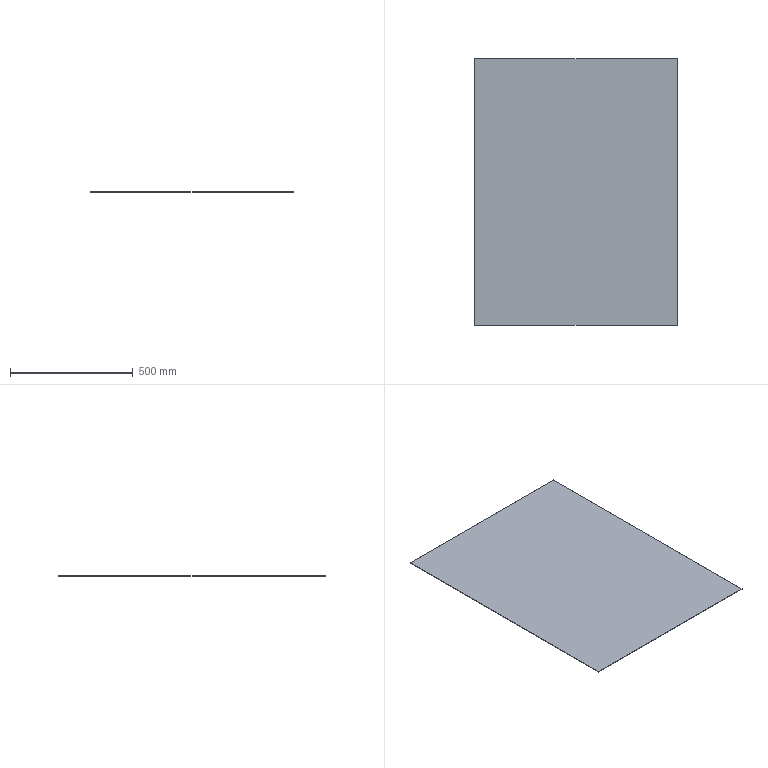Part | STEP file | Guide wheel mechanism revised.sldasm-Part-20 | 1 solid | 6 faces | box 825 x 1085 x 2 mm | volume 1790250 mm3 | plane 6
STEP:
#1=CARTESIAN_POINT('',(-412.5,812.5,-509.));
#2=VERTEX_POINT('',#1);
#3=CARTESIAN_POINT('',(-412.5,1897.5,-509.));
#4=VERTEX_POINT('',#3);
#5=CARTESIAN_POINT('',(-412.5,1897.5,-509.));
#6=DIRECTION('',(0.,1.,0.));
#7=VECTOR('',#6,1000.);
#8=LINE('',#5,#7);
#9=EDGE_CURVE('',#2,#4,#8,.T.);
#10=ORIENTED_EDGE('',*,*,#9,.T.);
#11=CARTESIAN_POINT('',(-412.5,1897.5,-511.));
#12=VERTEX_POINT('',#11);
#13=CARTESIAN_POINT('',(-412.5,1897.5,-511.));
#14=DIRECTION('',(0.,0.,1.));
#15=VECTOR('',#14,1000.);
#16=LINE('',#13,#15);
#17=EDGE_CURVE('',#12,#4,#16,.T.);
#18=ORIENTED_EDGE('',*,*,#17,.F.);
#19=CARTESIAN_POINT('',(-412.5,812.5,-511.));
#20=VERTEX_POINT('',#19);
#21=CARTESIAN_POINT('',(-412.5,1897.5,-511.));
#22=DIRECTION('',(0.,1.,0.));
#23=VECTOR('',#22,1000.);
#24=LINE('',#21,#23);
#25=EDGE_CURVE('',#20,#12,#24,.T.);
#26=ORIENTED_EDGE('',*,*,#25,.F.);
#27=CARTESIAN_POINT('',(-412.5,812.5,-511.));
#28=DIRECTION('',(0.,0.,1.));
#29=VECTOR('',#28,1000.);
#30=LINE('',#27,#29);
#31=EDGE_CURVE('',#20,#2,#30,.T.);
#32=ORIENTED_EDGE('',*,*,#31,.T.);
#33=EDGE_LOOP('',(#10,#18,#26,#32));
#34=FACE_OUTER_BOUND('',#33,.T.);
#35=CARTESIAN_POINT('',(-412.5,1897.5,-511.));
#36=DIRECTION('',(1.,0.,0.));
#37=DIRECTION('',(0.,1.,0.));
#38=AXIS2_PLACEMENT_3D('',#35,#36,#37);
#39=PLANE('',#38);
#40=ADVANCED_FACE('',(#34),#39,.F.);
#41=CARTESIAN_POINT('',(412.5,1897.5,-509.));
#42=VERTEX_POINT('',#41);
#43=CARTESIAN_POINT('',(-412.5,1897.5,-509.));
#44=DIRECTION('',(1.,0.,0.));
#45=VECTOR('',#44,1000.);
#46=LINE('',#43,#45);
#47=EDGE_CURVE('',#4,#42,#46,.T.);
#48=ORIENTED_EDGE('',*,*,#47,.T.);
#49=CARTESIAN_POINT('',(412.5,1897.5,-511.));
#50=VERTEX_POINT('',#49);
#51=CARTESIAN_POINT('',(412.5,1897.5,-511.));
#52=DIRECTION('',(0.,0.,1.));
#53=VECTOR('',#52,1000.);
#54=LINE('',#51,#53);
#55=EDGE_CURVE('',#50,#42,#54,.T.);
#56=ORIENTED_EDGE('',*,*,#55,.F.);
#57=CARTESIAN_POINT('',(-412.5,1897.5,-511.));
#58=DIRECTION('',(1.,0.,0.));
#59=VECTOR('',#58,1000.);
#60=LINE('',#57,#59);
#61=EDGE_CURVE('',#12,#50,#60,.T.);
#62=ORIENTED_EDGE('',*,*,#61,.F.);
#63=ORIENTED_EDGE('',*,*,#17,.T.);
#64=EDGE_LOOP('',(#48,#56,#62,#63));
#65=FACE_OUTER_BOUND('',#64,.T.);
#66=CARTESIAN_POINT('',(-412.5,1897.5,-511.));
#67=DIRECTION('',(0.,-1.,0.));
#68=DIRECTION('',(0.,0.,-1.));
#69=AXIS2_PLACEMENT_3D('',#66,#67,#68);
#70=PLANE('',#69);
#71=ADVANCED_FACE('',(#65),#70,.F.);
#72=CARTESIAN_POINT('',(412.5,812.5,-509.));
#73=VERTEX_POINT('',#72);
#74=CARTESIAN_POINT('',(412.5,1897.5,-509.));
#75=DIRECTION('',(0.,-1.,0.));
#76=VECTOR('',#75,1000.);
#77=LINE('',#74,#76);
#78=EDGE_CURVE('',#42,#73,#77,.T.);
#79=ORIENTED_EDGE('',*,*,#78,.T.);
#80=CARTESIAN_POINT('',(412.5,812.5,-511.));
#81=VERTEX_POINT('',#80);
#82=CARTESIAN_POINT('',(412.5,812.5,-511.));
#83=DIRECTION('',(0.,0.,1.));
#84=VECTOR('',#83,1000.);
#85=LINE('',#82,#84);
#86=EDGE_CURVE('',#81,#73,#85,.T.);
#87=ORIENTED_EDGE('',*,*,#86,.F.);
#88=CARTESIAN_POINT('',(412.5,1897.5,-511.));
#89=DIRECTION('',(0.,-1.,0.));
#90=VECTOR('',#89,1000.);
#91=LINE('',#88,#90);
#92=EDGE_CURVE('',#50,#81,#91,.T.);
#93=ORIENTED_EDGE('',*,*,#92,.F.);
#94=ORIENTED_EDGE('',*,*,#55,.T.);
#95=EDGE_LOOP('',(#79,#87,#93,#94));
#96=FACE_OUTER_BOUND('',#95,.T.);
#97=CARTESIAN_POINT('',(412.5,1897.5,-511.));
#98=DIRECTION('',(-1.,0.,0.));
#99=DIRECTION('',(0.,-1.,0.));
#100=AXIS2_PLACEMENT_3D('',#97,#98,#99);
#101=PLANE('',#100);
#102=ADVANCED_FACE('',(#96),#101,.F.);
#103=CARTESIAN_POINT('',(-412.5,812.5,-509.));
#104=DIRECTION('',(-1.,0.,0.));
#105=VECTOR('',#104,1000.);
#106=LINE('',#103,#105);
#107=EDGE_CURVE('',#73,#2,#106,.T.);
#108=ORIENTED_EDGE('',*,*,#107,.T.);
#109=ORIENTED_EDGE('',*,*,#31,.F.);
#110=CARTESIAN_POINT('',(-412.5,812.5,-511.));
#111=DIRECTION('',(-1.,0.,0.));
#112=VECTOR('',#111,1000.);
#113=LINE('',#110,#112);
#114=EDGE_CURVE('',#81,#20,#113,.T.);
#115=ORIENTED_EDGE('',*,*,#114,.F.);
#116=ORIENTED_EDGE('',*,*,#86,.T.);
#117=EDGE_LOOP('',(#108,#109,#115,#116));
#118=FACE_OUTER_BOUND('',#117,.T.);
#119=CARTESIAN_POINT('',(-412.5,812.5,-511.));
#120=DIRECTION('',(0.,1.,0.));
#121=DIRECTION('',(0.,0.,1.));
#122=AXIS2_PLACEMENT_3D('',#119,#120,#121);
#123=PLANE('',#122);
#124=ADVANCED_FACE('',(#118),#123,.F.);
#125=ORIENTED_EDGE('',*,*,#25,.T.);
#126=ORIENTED_EDGE('',*,*,#61,.T.);
#127=ORIENTED_EDGE('',*,*,#92,.T.);
#128=ORIENTED_EDGE('',*,*,#114,.T.);
#129=EDGE_LOOP('',(#125,#126,#127,#128));
#130=FACE_OUTER_BOUND('',#129,.T.);
#131=CARTESIAN_POINT('',(0.,0.,-511.));
#132=DIRECTION('',(0.,0.,1.));
#133=DIRECTION('',(1.,0.,0.));
#134=AXIS2_PLACEMENT_3D('',#131,#132,#133);
#135=PLANE('',#134);
#136=ADVANCED_FACE('',(#130),#135,.F.);
#137=ORIENTED_EDGE('',*,*,#9,.F.);
#138=ORIENTED_EDGE('',*,*,#107,.F.);
#139=ORIENTED_EDGE('',*,*,#78,.F.);
#140=ORIENTED_EDGE('',*,*,#47,.F.);
#141=EDGE_LOOP('',(#137,#138,#139,#140));
#142=FACE_OUTER_BOUND('',#141,.T.);
#143=CARTESIAN_POINT('',(0.,0.,-509.));
#144=DIRECTION('',(0.,0.,1.));
#145=DIRECTION('',(1.,0.,0.));
#146=AXIS2_PLACEMENT_3D('',#143,#144,#145);
#147=PLANE('',#146);
#148=ADVANCED_FACE('',(#142),#147,.T.);
#149=CLOSED_SHELL('',(#40,#71,#102,#124,#136,#148));
#150=MANIFOLD_SOLID_BREP('',#149);
#151=CARTESIAN_POINT('',(0.,0.,0.));
#152=DIRECTION('',(0.,0.,1.));
#153=DIRECTION('',(1.,0.,0.));
#154=AXIS2_PLACEMENT_3D('',#151,#152,#153);
#155=(LENGTH_UNIT()NAMED_UNIT(*)SI_UNIT(.MILLI.,.METRE.));
#156=UNCERTAINTY_MEASURE_WITH_UNIT(LENGTH_MEASURE(0.00001),#155,'','');
#157=(NAMED_UNIT(*)PLANE_ANGLE_UNIT()SI_UNIT($,.RADIAN.));
#158=(NAMED_UNIT(*)SI_UNIT($,.STERADIAN.)SOLID_ANGLE_UNIT());
#159=(GEOMETRIC_REPRESENTATION_CONTEXT(3)GLOBAL_UNCERTAINTY_ASSIGNED_CONTEXT((#156))GLOBAL_UNIT_ASSIGNED_CONTEXT((#155,#157,#158))REPRESENTATION_CONTEXT('',''));
#160=ADVANCED_BREP_SHAPE_REPRESENTATION('',(#150,#154),#159);